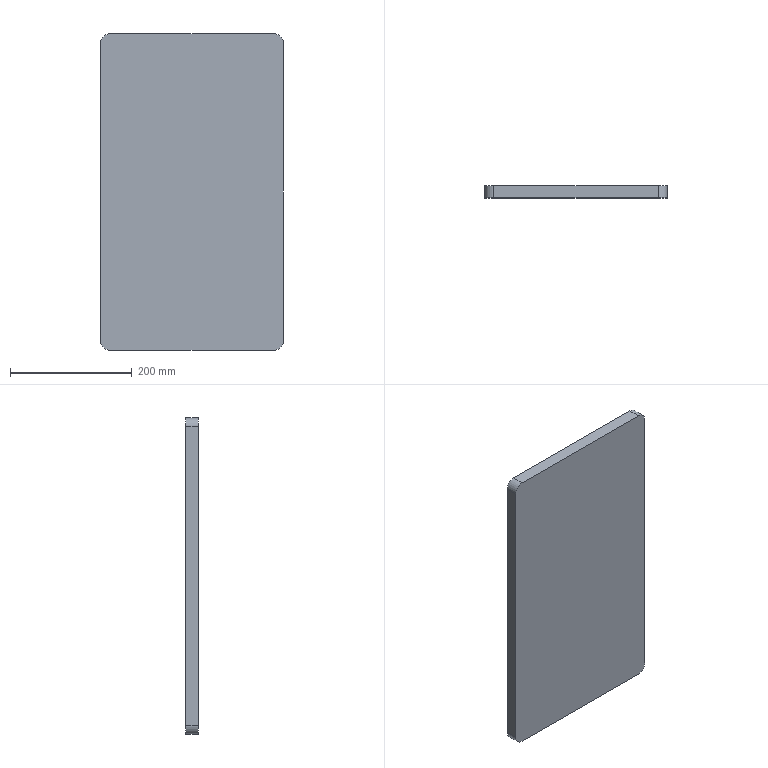Part | SolidWorks | features Extrusion 1 | 1 solid | 10 faces | box 300 x 20 x 520 mm | volume 3116137 mm3 | plane 6 | cylinder 4 | commonest cylinder face diameters 30 x4
STEP:
#1=CARTESIAN_POINT('',(-135.,0.,-260.));
#2=VERTEX_POINT('',#1);
#3=CARTESIAN_POINT('',(-150.,0.,-245.));
#4=VERTEX_POINT('',#3);
#5=CARTESIAN_POINT('',(-135.,0.,-245.));
#6=DIRECTION('',(0.,1.,0.));
#7=DIRECTION('',(0.,0.,1.));
#8=AXIS2_PLACEMENT_3D('',#5,#6,#7);
#9=CIRCLE('',#8,15.);
#10=EDGE_CURVE('',#2,#4,#9,.T.);
#11=ORIENTED_EDGE('',*,*,#10,.T.);
#12=CARTESIAN_POINT('',(-150.,20.,-245.));
#13=VERTEX_POINT('',#12);
#14=CARTESIAN_POINT('',(-150.,20.,-245.));
#15=DIRECTION('',(0.,-1.,0.));
#16=VECTOR('',#15,1000.);
#17=LINE('',#14,#16);
#18=EDGE_CURVE('',#13,#4,#17,.T.);
#19=ORIENTED_EDGE('',*,*,#18,.F.);
#20=CARTESIAN_POINT('',(-135.,20.,-260.));
#21=VERTEX_POINT('',#20);
#22=CARTESIAN_POINT('',(-135.,20.,-245.));
#23=DIRECTION('',(0.,1.,0.));
#24=DIRECTION('',(0.,0.,1.));
#25=AXIS2_PLACEMENT_3D('',#22,#23,#24);
#26=CIRCLE('',#25,15.);
#27=EDGE_CURVE('',#21,#13,#26,.T.);
#28=ORIENTED_EDGE('',*,*,#27,.F.);
#29=CARTESIAN_POINT('',(-135.,20.,-260.));
#30=DIRECTION('',(0.,-1.,0.));
#31=VECTOR('',#30,1000.);
#32=LINE('',#29,#31);
#33=EDGE_CURVE('',#21,#2,#32,.T.);
#34=ORIENTED_EDGE('',*,*,#33,.T.);
#35=EDGE_LOOP('',(#11,#19,#28,#34));
#36=FACE_OUTER_BOUND('',#35,.T.);
#37=CARTESIAN_POINT('',(-135.,20.,-245.));
#38=DIRECTION('',(0.,-1.,0.));
#39=DIRECTION('',(0.,0.,-1.));
#40=AXIS2_PLACEMENT_3D('',#37,#38,#39);
#41=CYLINDRICAL_SURFACE('',#40,15.);
#42=ADVANCED_FACE('',(#36),#41,.T.);
#43=CARTESIAN_POINT('',(-150.,0.,245.));
#44=VERTEX_POINT('',#43);
#45=CARTESIAN_POINT('',(-150.,0.,-245.));
#46=DIRECTION('',(0.,0.,1.));
#47=VECTOR('',#46,1000.);
#48=LINE('',#45,#47);
#49=EDGE_CURVE('',#4,#44,#48,.T.);
#50=ORIENTED_EDGE('',*,*,#49,.T.);
#51=CARTESIAN_POINT('',(-150.,20.,245.));
#52=VERTEX_POINT('',#51);
#53=CARTESIAN_POINT('',(-150.,20.,245.));
#54=DIRECTION('',(0.,-1.,0.));
#55=VECTOR('',#54,1000.);
#56=LINE('',#53,#55);
#57=EDGE_CURVE('',#52,#44,#56,.T.);
#58=ORIENTED_EDGE('',*,*,#57,.F.);
#59=CARTESIAN_POINT('',(-150.,20.,-245.));
#60=DIRECTION('',(0.,0.,1.));
#61=VECTOR('',#60,1000.);
#62=LINE('',#59,#61);
#63=EDGE_CURVE('',#13,#52,#62,.T.);
#64=ORIENTED_EDGE('',*,*,#63,.F.);
#65=ORIENTED_EDGE('',*,*,#18,.T.);
#66=EDGE_LOOP('',(#50,#58,#64,#65));
#67=FACE_OUTER_BOUND('',#66,.T.);
#68=CARTESIAN_POINT('',(-150.,20.,-245.));
#69=DIRECTION('',(1.,0.,0.));
#70=DIRECTION('',(0.,0.,-1.));
#71=AXIS2_PLACEMENT_3D('',#68,#69,#70);
#72=PLANE('',#71);
#73=ADVANCED_FACE('',(#67),#72,.F.);
#74=CARTESIAN_POINT('',(-135.,0.,260.));
#75=VERTEX_POINT('',#74);
#76=CARTESIAN_POINT('',(-135.,0.,245.));
#77=DIRECTION('',(0.,1.,0.));
#78=DIRECTION('',(0.,0.,-1.));
#79=AXIS2_PLACEMENT_3D('',#76,#77,#78);
#80=CIRCLE('',#79,15.);
#81=EDGE_CURVE('',#44,#75,#80,.T.);
#82=ORIENTED_EDGE('',*,*,#81,.T.);
#83=CARTESIAN_POINT('',(-135.,20.,260.));
#84=VERTEX_POINT('',#83);
#85=CARTESIAN_POINT('',(-135.,20.,260.));
#86=DIRECTION('',(0.,-1.,0.));
#87=VECTOR('',#86,1000.);
#88=LINE('',#85,#87);
#89=EDGE_CURVE('',#84,#75,#88,.T.);
#90=ORIENTED_EDGE('',*,*,#89,.F.);
#91=CARTESIAN_POINT('',(-135.,20.,245.));
#92=DIRECTION('',(0.,1.,0.));
#93=DIRECTION('',(0.,0.,-1.));
#94=AXIS2_PLACEMENT_3D('',#91,#92,#93);
#95=CIRCLE('',#94,15.);
#96=EDGE_CURVE('',#52,#84,#95,.T.);
#97=ORIENTED_EDGE('',*,*,#96,.F.);
#98=ORIENTED_EDGE('',*,*,#57,.T.);
#99=EDGE_LOOP('',(#82,#90,#97,#98));
#100=FACE_OUTER_BOUND('',#99,.T.);
#101=CARTESIAN_POINT('',(-135.,20.,245.));
#102=DIRECTION('',(0.,-1.,0.));
#103=DIRECTION('',(0.,0.,-1.));
#104=AXIS2_PLACEMENT_3D('',#101,#102,#103);
#105=CYLINDRICAL_SURFACE('',#104,15.);
#106=ADVANCED_FACE('',(#100),#105,.T.);
#107=CARTESIAN_POINT('',(135.,0.,260.));
#108=VERTEX_POINT('',#107);
#109=CARTESIAN_POINT('',(135.,0.,260.));
#110=DIRECTION('',(1.,0.,0.));
#111=VECTOR('',#110,1000.);
#112=LINE('',#109,#111);
#113=EDGE_CURVE('',#75,#108,#112,.T.);
#114=ORIENTED_EDGE('',*,*,#113,.T.);
#115=CARTESIAN_POINT('',(135.,20.,260.));
#116=VERTEX_POINT('',#115);
#117=CARTESIAN_POINT('',(135.,20.,260.));
#118=DIRECTION('',(0.,-1.,0.));
#119=VECTOR('',#118,1000.);
#120=LINE('',#117,#119);
#121=EDGE_CURVE('',#116,#108,#120,.T.);
#122=ORIENTED_EDGE('',*,*,#121,.F.);
#123=CARTESIAN_POINT('',(135.,20.,260.));
#124=DIRECTION('',(1.,0.,0.));
#125=VECTOR('',#124,1000.);
#126=LINE('',#123,#125);
#127=EDGE_CURVE('',#84,#116,#126,.T.);
#128=ORIENTED_EDGE('',*,*,#127,.F.);
#129=ORIENTED_EDGE('',*,*,#89,.T.);
#130=EDGE_LOOP('',(#114,#122,#128,#129));
#131=FACE_OUTER_BOUND('',#130,.T.);
#132=CARTESIAN_POINT('',(135.,20.,260.));
#133=DIRECTION('',(0.,0.,-1.));
#134=DIRECTION('',(-1.,0.,0.));
#135=AXIS2_PLACEMENT_3D('',#132,#133,#134);
#136=PLANE('',#135);
#137=ADVANCED_FACE('',(#131),#136,.F.);
#138=CARTESIAN_POINT('',(150.,0.,245.));
#139=VERTEX_POINT('',#138);
#140=CARTESIAN_POINT('',(135.,0.,245.));
#141=DIRECTION('',(0.,1.,0.));
#142=DIRECTION('',(0.,0.,1.));
#143=AXIS2_PLACEMENT_3D('',#140,#141,#142);
#144=CIRCLE('',#143,15.);
#145=EDGE_CURVE('',#108,#139,#144,.T.);
#146=ORIENTED_EDGE('',*,*,#145,.T.);
#147=CARTESIAN_POINT('',(150.,20.,245.));
#148=VERTEX_POINT('',#147);
#149=CARTESIAN_POINT('',(150.,20.,245.));
#150=DIRECTION('',(0.,-1.,0.));
#151=VECTOR('',#150,1000.);
#152=LINE('',#149,#151);
#153=EDGE_CURVE('',#148,#139,#152,.T.);
#154=ORIENTED_EDGE('',*,*,#153,.F.);
#155=CARTESIAN_POINT('',(135.,20.,245.));
#156=DIRECTION('',(0.,1.,0.));
#157=DIRECTION('',(0.,0.,1.));
#158=AXIS2_PLACEMENT_3D('',#155,#156,#157);
#159=CIRCLE('',#158,15.);
#160=EDGE_CURVE('',#116,#148,#159,.T.);
#161=ORIENTED_EDGE('',*,*,#160,.F.);
#162=ORIENTED_EDGE('',*,*,#121,.T.);
#163=EDGE_LOOP('',(#146,#154,#161,#162));
#164=FACE_OUTER_BOUND('',#163,.T.);
#165=CARTESIAN_POINT('',(135.,20.,245.));
#166=DIRECTION('',(0.,-1.,0.));
#167=DIRECTION('',(0.,0.,-1.));
#168=AXIS2_PLACEMENT_3D('',#165,#166,#167);
#169=CYLINDRICAL_SURFACE('',#168,15.);
#170=ADVANCED_FACE('',(#164),#169,.T.);
#171=CARTESIAN_POINT('',(150.,0.,-245.));
#172=VERTEX_POINT('',#171);
#173=CARTESIAN_POINT('',(150.,0.,-245.));
#174=DIRECTION('',(0.,0.,-1.));
#175=VECTOR('',#174,1000.);
#176=LINE('',#173,#175);
#177=EDGE_CURVE('',#139,#172,#176,.T.);
#178=ORIENTED_EDGE('',*,*,#177,.T.);
#179=CARTESIAN_POINT('',(150.,20.,-245.));
#180=VERTEX_POINT('',#179);
#181=CARTESIAN_POINT('',(150.,20.,-245.));
#182=DIRECTION('',(0.,-1.,0.));
#183=VECTOR('',#182,1000.);
#184=LINE('',#181,#183);
#185=EDGE_CURVE('',#180,#172,#184,.T.);
#186=ORIENTED_EDGE('',*,*,#185,.F.);
#187=CARTESIAN_POINT('',(150.,20.,-245.));
#188=DIRECTION('',(0.,0.,-1.));
#189=VECTOR('',#188,1000.);
#190=LINE('',#187,#189);
#191=EDGE_CURVE('',#148,#180,#190,.T.);
#192=ORIENTED_EDGE('',*,*,#191,.F.);
#193=ORIENTED_EDGE('',*,*,#153,.T.);
#194=EDGE_LOOP('',(#178,#186,#192,#193));
#195=FACE_OUTER_BOUND('',#194,.T.);
#196=CARTESIAN_POINT('',(150.,20.,-245.));
#197=DIRECTION('',(-1.,0.,0.));
#198=DIRECTION('',(0.,0.,1.));
#199=AXIS2_PLACEMENT_3D('',#196,#197,#198);
#200=PLANE('',#199);
#201=ADVANCED_FACE('',(#195),#200,.F.);
#202=CARTESIAN_POINT('',(135.,0.,-260.));
#203=VERTEX_POINT('',#202);
#204=CARTESIAN_POINT('',(135.,0.,-245.));
#205=DIRECTION('',(0.,1.,0.));
#206=DIRECTION('',(0.,0.,-1.));
#207=AXIS2_PLACEMENT_3D('',#204,#205,#206);
#208=CIRCLE('',#207,15.);
#209=EDGE_CURVE('',#172,#203,#208,.T.);
#210=ORIENTED_EDGE('',*,*,#209,.T.);
#211=CARTESIAN_POINT('',(135.,20.,-260.));
#212=VERTEX_POINT('',#211);
#213=CARTESIAN_POINT('',(135.,20.,-260.));
#214=DIRECTION('',(0.,-1.,0.));
#215=VECTOR('',#214,1000.);
#216=LINE('',#213,#215);
#217=EDGE_CURVE('',#212,#203,#216,.T.);
#218=ORIENTED_EDGE('',*,*,#217,.F.);
#219=CARTESIAN_POINT('',(135.,20.,-245.));
#220=DIRECTION('',(0.,1.,0.));
#221=DIRECTION('',(0.,0.,-1.));
#222=AXIS2_PLACEMENT_3D('',#219,#220,#221);
#223=CIRCLE('',#222,15.);
#224=EDGE_CURVE('',#180,#212,#223,.T.);
#225=ORIENTED_EDGE('',*,*,#224,.F.);
#226=ORIENTED_EDGE('',*,*,#185,.T.);
#227=EDGE_LOOP('',(#210,#218,#225,#226));
#228=FACE_OUTER_BOUND('',#227,.T.);
#229=CARTESIAN_POINT('',(135.,20.,-245.));
#230=DIRECTION('',(0.,-1.,0.));
#231=DIRECTION('',(0.,0.,-1.));
#232=AXIS2_PLACEMENT_3D('',#229,#230,#231);
#233=CYLINDRICAL_SURFACE('',#232,15.);
#234=ADVANCED_FACE('',(#228),#233,.T.);
#235=CARTESIAN_POINT('',(135.,0.,-260.));
#236=DIRECTION('',(-1.,0.,0.));
#237=VECTOR('',#236,1000.);
#238=LINE('',#235,#237);
#239=EDGE_CURVE('',#203,#2,#238,.T.);
#240=ORIENTED_EDGE('',*,*,#239,.T.);
#241=ORIENTED_EDGE('',*,*,#33,.F.);
#242=CARTESIAN_POINT('',(135.,20.,-260.));
#243=DIRECTION('',(-1.,0.,0.));
#244=VECTOR('',#243,1000.);
#245=LINE('',#242,#244);
#246=EDGE_CURVE('',#212,#21,#245,.T.);
#247=ORIENTED_EDGE('',*,*,#246,.F.);
#248=ORIENTED_EDGE('',*,*,#217,.T.);
#249=EDGE_LOOP('',(#240,#241,#247,#248));
#250=FACE_OUTER_BOUND('',#249,.T.);
#251=CARTESIAN_POINT('',(135.,20.,-260.));
#252=DIRECTION('',(0.,0.,1.));
#253=DIRECTION('',(1.,0.,0.));
#254=AXIS2_PLACEMENT_3D('',#251,#252,#253);
#255=PLANE('',#254);
#256=ADVANCED_FACE('',(#250),#255,.F.);
#257=ORIENTED_EDGE('',*,*,#27,.T.);
#258=ORIENTED_EDGE('',*,*,#63,.T.);
#259=ORIENTED_EDGE('',*,*,#96,.T.);
#260=ORIENTED_EDGE('',*,*,#127,.T.);
#261=ORIENTED_EDGE('',*,*,#160,.T.);
#262=ORIENTED_EDGE('',*,*,#191,.T.);
#263=ORIENTED_EDGE('',*,*,#224,.T.);
#264=ORIENTED_EDGE('',*,*,#246,.T.);
#265=EDGE_LOOP('',(#257,#258,#259,#260,#261,#262,#263,#264));
#266=FACE_OUTER_BOUND('',#265,.T.);
#267=CARTESIAN_POINT('',(-135.,20.,-245.));
#268=DIRECTION('',(0.,1.,0.));
#269=DIRECTION('',(0.,0.,1.));
#270=AXIS2_PLACEMENT_3D('',#267,#268,#269);
#271=PLANE('',#270);
#272=ADVANCED_FACE('',(#266),#271,.T.);
#273=ORIENTED_EDGE('',*,*,#10,.F.);
#274=ORIENTED_EDGE('',*,*,#239,.F.);
#275=ORIENTED_EDGE('',*,*,#209,.F.);
#276=ORIENTED_EDGE('',*,*,#177,.F.);
#277=ORIENTED_EDGE('',*,*,#145,.F.);
#278=ORIENTED_EDGE('',*,*,#113,.F.);
#279=ORIENTED_EDGE('',*,*,#81,.F.);
#280=ORIENTED_EDGE('',*,*,#49,.F.);
#281=EDGE_LOOP('',(#273,#274,#275,#276,#277,#278,#279,#280));
#282=FACE_OUTER_BOUND('',#281,.T.);
#283=CARTESIAN_POINT('',(-135.,0.,-245.));
#284=DIRECTION('',(0.,1.,0.));
#285=DIRECTION('',(0.,0.,1.));
#286=AXIS2_PLACEMENT_3D('',#283,#284,#285);
#287=PLANE('',#286);
#288=ADVANCED_FACE('',(#282),#287,.F.);
#289=CLOSED_SHELL('',(#42,#73,#106,#137,#170,#201,#234,#256,#272,#288));
#290=MANIFOLD_SOLID_BREP('',#289);
#291=CARTESIAN_POINT('',(0.,0.,0.));
#292=DIRECTION('',(0.,0.,1.));
#293=DIRECTION('',(1.,0.,0.));
#294=AXIS2_PLACEMENT_3D('',#291,#292,#293);
#295=(LENGTH_UNIT()NAMED_UNIT(*)SI_UNIT(.MILLI.,.METRE.));
#296=UNCERTAINTY_MEASURE_WITH_UNIT(LENGTH_MEASURE(0.00001),#295,'','');
#297=(NAMED_UNIT(*)PLANE_ANGLE_UNIT()SI_UNIT($,.RADIAN.));
#298=(NAMED_UNIT(*)SI_UNIT($,.STERADIAN.)SOLID_ANGLE_UNIT());
#299=(GEOMETRIC_REPRESENTATION_CONTEXT(3)GLOBAL_UNCERTAINTY_ASSIGNED_CONTEXT((#296))GLOBAL_UNIT_ASSIGNED_CONTEXT((#295,#297,#298))REPRESENTATION_CONTEXT('',''));
#300=ADVANCED_BREP_SHAPE_REPRESENTATION('',(#290,#294),#299);